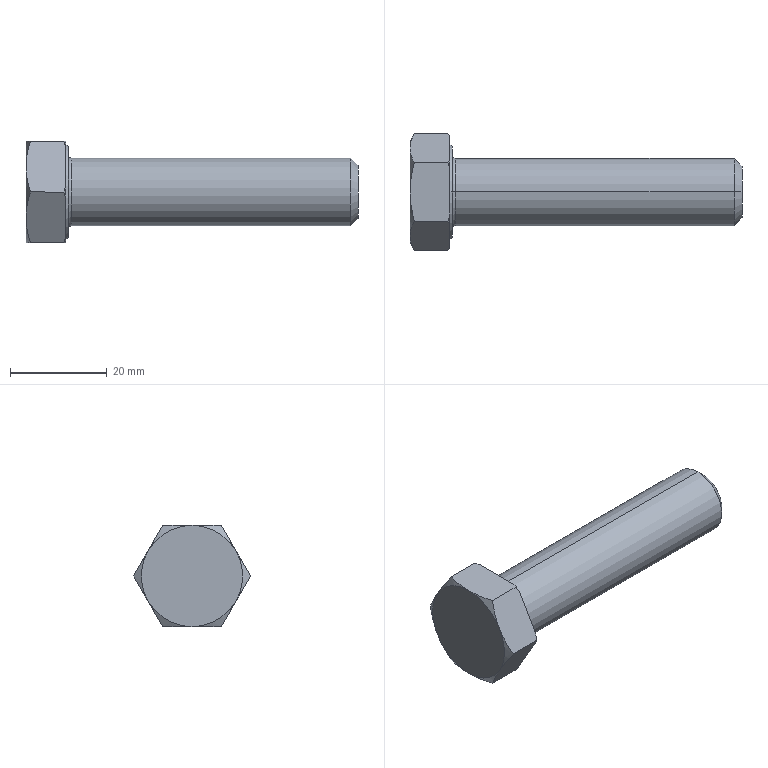Part | SolidWorks | features RevCut 4, Revolution 2, Chamfer 1, Extrusion 1, LPattern 1 | 1 solid | 30 faces | box 68.8 x 24.249 x 21 mm | volume 12486 mm3 | cone 16 | plane 10 | cylinder 2 | torus 2 | commonest cylinder face diameters 14 x2
STEP:
#1=CARTESIAN_POINT('',(9.4,0.,7.));
#2=VERTEX_POINT('',#1);
#3=CARTESIAN_POINT('',(9.4,0.,-7.));
#4=VERTEX_POINT('',#3);
#5=CARTESIAN_POINT('',(9.4,0.,0.));
#6=DIRECTION('',(-1.,0.,0.));
#7=DIRECTION('',(0.,0.,1.));
#8=AXIS2_PLACEMENT_3D('',#5,#6,#7);
#9=CIRCLE('',#8,7.);
#10=EDGE_CURVE('',#2,#4,#9,.T.);
#11=ORIENTED_EDGE('',*,*,#10,.F.);
#12=CARTESIAN_POINT('',(67.2,0.,7.));
#13=VERTEX_POINT('',#12);
#14=CARTESIAN_POINT('',(0.,0.,7.));
#15=DIRECTION('',(1.,0.,0.));
#16=VECTOR('',#15,1000.);
#17=LINE('',#14,#16);
#18=EDGE_CURVE('',#2,#13,#17,.T.);
#19=ORIENTED_EDGE('',*,*,#18,.T.);
#20=CARTESIAN_POINT('',(67.2,0.,-7.));
#21=VERTEX_POINT('',#20);
#22=CARTESIAN_POINT('',(67.2,0.,0.));
#23=DIRECTION('',(-1.,0.,0.));
#24=DIRECTION('',(0.,0.,-1.));
#25=AXIS2_PLACEMENT_3D('',#22,#23,#24);
#26=CIRCLE('',#25,7.);
#27=EDGE_CURVE('',#13,#21,#26,.T.);
#28=ORIENTED_EDGE('',*,*,#27,.T.);
#29=CARTESIAN_POINT('',(0.,0.,-7.));
#30=DIRECTION('',(1.,0.,0.));
#31=VECTOR('',#30,1000.);
#32=LINE('',#29,#31);
#33=EDGE_CURVE('',#4,#21,#32,.T.);
#34=ORIENTED_EDGE('',*,*,#33,.F.);
#35=EDGE_LOOP('',(#11,#19,#28,#34));
#36=FACE_OUTER_BOUND('',#35,.T.);
#37=CARTESIAN_POINT('',(0.,0.,0.));
#38=DIRECTION('',(1.,0.,0.));
#39=DIRECTION('',(0.,0.,-1.));
#40=AXIS2_PLACEMENT_3D('',#37,#38,#39);
#41=CYLINDRICAL_SURFACE('',#40,7.);
#42=ADVANCED_FACE('',(#36),#41,.T.);
#43=CARTESIAN_POINT('',(68.8,0.,-5.4));
#44=VERTEX_POINT('',#43);
#45=CARTESIAN_POINT('',(68.8,0.,5.4));
#46=VERTEX_POINT('',#45);
#47=CARTESIAN_POINT('',(68.8,0.,0.));
#48=DIRECTION('',(1.,0.,0.));
#49=DIRECTION('',(0.,0.,-1.));
#50=AXIS2_PLACEMENT_3D('',#47,#48,#49);
#51=CIRCLE('',#50,5.4);
#52=EDGE_CURVE('',#44,#46,#51,.T.);
#53=ORIENTED_EDGE('',*,*,#52,.F.);
#54=CARTESIAN_POINT('',(68.8,0.,-5.4));
#55=DIRECTION('',(-0.7071,0.,-0.7071));
#56=VECTOR('',#55,1000.);
#57=LINE('',#54,#56);
#58=EDGE_CURVE('',#44,#21,#57,.T.);
#59=ORIENTED_EDGE('',*,*,#58,.T.);
#60=ORIENTED_EDGE('',*,*,#27,.F.);
#61=CARTESIAN_POINT('',(68.8,0.,5.4));
#62=DIRECTION('',(-0.7071,0.,0.7071));
#63=VECTOR('',#62,1000.);
#64=LINE('',#61,#63);
#65=EDGE_CURVE('',#46,#13,#64,.T.);
#66=ORIENTED_EDGE('',*,*,#65,.F.);
#67=EDGE_LOOP('',(#53,#59,#60,#66));
#68=FACE_OUTER_BOUND('',#67,.T.);
#69=CARTESIAN_POINT('',(68.8,0.,0.));
#70=DIRECTION('',(-1.,0.,0.));
#71=DIRECTION('',(0.,0.,1.));
#72=AXIS2_PLACEMENT_3D('',#69,#70,#71);
#73=CONICAL_SURFACE('',#72,5.4,0.7854);
#74=ADVANCED_FACE('',(#68),#73,.T.);
#75=CARTESIAN_POINT('',(8.8,0.,-7.6));
#76=VERTEX_POINT('',#75);
#77=CARTESIAN_POINT('',(8.8,0.,7.6));
#78=VERTEX_POINT('',#77);
#79=CARTESIAN_POINT('',(8.8,0.,0.));
#80=DIRECTION('',(-1.,0.,0.));
#81=DIRECTION('',(0.,0.,1.));
#82=AXIS2_PLACEMENT_3D('',#79,#80,#81);
#83=CIRCLE('',#82,7.6);
#84=EDGE_CURVE('',#76,#78,#83,.T.);
#85=ORIENTED_EDGE('',*,*,#84,.F.);
#86=CARTESIAN_POINT('',(9.4,0.,-7.6));
#87=DIRECTION('',(0.,1.,0.));
#88=DIRECTION('',(0.,0.,1.));
#89=AXIS2_PLACEMENT_3D('',#86,#87,#88);
#90=CIRCLE('',#89,0.6);
#91=EDGE_CURVE('',#76,#4,#90,.T.);
#92=ORIENTED_EDGE('',*,*,#91,.T.);
#93=CARTESIAN_POINT('',(9.4,0.,0.));
#94=DIRECTION('',(-1.,0.,0.));
#95=DIRECTION('',(0.,0.,1.));
#96=AXIS2_PLACEMENT_3D('',#93,#94,#95);
#97=CIRCLE('',#96,7.);
#98=EDGE_CURVE('',#4,#2,#97,.T.);
#99=ORIENTED_EDGE('',*,*,#98,.T.);
#100=CARTESIAN_POINT('',(9.4,0.,7.6));
#101=DIRECTION('',(0.,-1.,0.));
#102=DIRECTION('',(1.,0.,0.));
#103=AXIS2_PLACEMENT_3D('',#100,#101,#102);
#104=CIRCLE('',#103,0.6);
#105=EDGE_CURVE('',#78,#2,#104,.T.);
#106=ORIENTED_EDGE('',*,*,#105,.F.);
#107=EDGE_LOOP('',(#85,#92,#99,#106));
#108=FACE_OUTER_BOUND('',#107,.T.);
#109=CARTESIAN_POINT('',(9.4,0.,0.));
#110=DIRECTION('',(-1.,0.,0.));
#111=DIRECTION('',(0.,0.,1.));
#112=AXIS2_PLACEMENT_3D('',#109,#110,#111);
#113=TOROIDAL_SURFACE('',#112,7.6,0.6);
#114=ADVANCED_FACE('',(#108),#113,.F.);
#115=CARTESIAN_POINT('',(8.8,0.,9.517));
#116=VERTEX_POINT('',#115);
#117=CARTESIAN_POINT('',(8.8,0.,-9.517));
#118=VERTEX_POINT('',#117);
#119=CARTESIAN_POINT('',(8.8,0.,0.));
#120=DIRECTION('',(-1.,0.,0.));
#121=DIRECTION('',(0.,0.,1.));
#122=AXIS2_PLACEMENT_3D('',#119,#120,#121);
#123=CIRCLE('',#122,9.517);
#124=EDGE_CURVE('',#116,#118,#123,.T.);
#125=ORIENTED_EDGE('',*,*,#124,.T.);
#126=CARTESIAN_POINT('',(8.2,0.,-9.864));
#127=VERTEX_POINT('',#126);
#128=CARTESIAN_POINT('',(8.2,0.,-9.864));
#129=DIRECTION('',(-0.866,0.,-0.5));
#130=VECTOR('',#129,1000.);
#131=LINE('',#128,#130);
#132=EDGE_CURVE('',#118,#127,#131,.T.);
#133=ORIENTED_EDGE('',*,*,#132,.T.);
#134=CARTESIAN_POINT('',(8.2,0.,9.864));
#135=VERTEX_POINT('',#134);
#136=CARTESIAN_POINT('',(8.2,0.,0.));
#137=DIRECTION('',(-1.,0.,0.));
#138=DIRECTION('',(0.,0.,1.));
#139=AXIS2_PLACEMENT_3D('',#136,#137,#138);
#140=CIRCLE('',#139,9.864);
#141=EDGE_CURVE('',#135,#127,#140,.T.);
#142=ORIENTED_EDGE('',*,*,#141,.F.);
#143=CARTESIAN_POINT('',(8.2,0.,9.864));
#144=DIRECTION('',(-0.866,0.,0.5));
#145=VECTOR('',#144,1000.);
#146=LINE('',#143,#145);
#147=EDGE_CURVE('',#116,#135,#146,.T.);
#148=ORIENTED_EDGE('',*,*,#147,.F.);
#149=EDGE_LOOP('',(#125,#133,#142,#148));
#150=FACE_OUTER_BOUND('',#149,.T.);
#151=CARTESIAN_POINT('',(8.2,0.,0.));
#152=DIRECTION('',(-1.,0.,0.));
#153=DIRECTION('',(0.,0.,1.));
#154=AXIS2_PLACEMENT_3D('',#151,#152,#153);
#155=CONICAL_SURFACE('',#154,9.864,0.5236);
#156=ADVANCED_FACE('',(#150),#155,.T.);
#157=ORIENTED_EDGE('',*,*,#124,.F.);
#158=CARTESIAN_POINT('',(8.8,0.,0.));
#159=DIRECTION('',(-1.,0.,0.));
#160=DIRECTION('',(0.,0.,1.));
#161=AXIS2_PLACEMENT_3D('',#158,#159,#160);
#162=CIRCLE('',#161,9.517);
#163=EDGE_CURVE('',#118,#116,#162,.T.);
#164=ORIENTED_EDGE('',*,*,#163,.F.);
#165=EDGE_LOOP('',(#157,#164));
#166=FACE_OUTER_BOUND('',#165,.T.);
#167=CARTESIAN_POINT('',(8.8,0.,0.));
#168=DIRECTION('',(-1.,0.,0.));
#169=DIRECTION('',(0.,0.,1.));
#170=AXIS2_PLACEMENT_3D('',#167,#168,#169);
#171=CIRCLE('',#170,7.6);
#172=EDGE_CURVE('',#78,#76,#171,.T.);
#173=ORIENTED_EDGE('',*,*,#172,.T.);
#174=ORIENTED_EDGE('',*,*,#84,.T.);
#175=EDGE_LOOP('',(#173,#174));
#176=FACE_BOUND('',#175,.T.);
#177=CARTESIAN_POINT('',(8.8,12.124,0.));
#178=DIRECTION('',(1.,0.,0.));
#179=DIRECTION('',(0.,0.,-1.));
#180=AXIS2_PLACEMENT_3D('',#177,#178,#179);
#181=PLANE('',#180);
#182=ADVANCED_FACE('',(#166,#176),#181,.T.);
#183=CARTESIAN_POINT('',(8.2,6.7,-9.395));
#184=VERTEX_POINT('',#183);
#185=CARTESIAN_POINT('',(8.2,11.486,-1.105));
#186=VERTEX_POINT('',#185);
#187=CARTESIAN_POINT('',(8.2,6.062,-10.5));
#188=DIRECTION('',(0.,0.5,0.866));
#189=VECTOR('',#188,1000.);
#190=LINE('',#187,#189);
#191=EDGE_CURVE('',#184,#186,#190,.T.);
#192=ORIENTED_EDGE('',*,*,#191,.F.);
#193=CARTESIAN_POINT('',(7.862,6.062,-10.5));
#194=VERTEX_POINT('',#193);
#195=CARTESIAN_POINT('',(7.862,6.062,-10.5));
#196=CARTESIAN_POINT('',(7.985,6.274,-10.133));
#197=CARTESIAN_POINT('',(8.098,6.487,-9.764));
#198=CARTESIAN_POINT('',(8.2,6.7,-9.395));
#199=B_SPLINE_CURVE_WITH_KNOTS('',3,(#195,#196,#197,#198),.UNSPECIFIED.,.F.,.F.,(4,4),(0.000000238,0.001312),.UNSPECIFIED.);
#200=EDGE_CURVE('',#194,#184,#199,.T.);
#201=ORIENTED_EDGE('',*,*,#200,.F.);
#202=CARTESIAN_POINT('',(0.9378,6.062,-10.5));
#203=VERTEX_POINT('',#202);
#204=CARTESIAN_POINT('',(8.8,6.062,-10.5));
#205=DIRECTION('',(-1.,0.,0.));
#206=VECTOR('',#205,1000.);
#207=LINE('',#204,#206);
#208=EDGE_CURVE('',#194,#203,#207,.T.);
#209=ORIENTED_EDGE('',*,*,#208,.T.);
#210=CARTESIAN_POINT('',(0.,9.093,-5.25));
#211=VERTEX_POINT('',#210);
#212=CARTESIAN_POINT('',(0.,9.093,-5.25));
#213=CARTESIAN_POINT('',(0.,8.836,-5.696));
#214=CARTESIAN_POINT('',(0.02217,8.578,-6.143));
#215=CARTESIAN_POINT('',(0.1079,8.066,-7.028));
#216=CARTESIAN_POINT('',(0.1715,7.813,-7.468));
#217=CARTESIAN_POINT('',(0.4165,7.056,-8.779));
#218=CARTESIAN_POINT('',(0.6523,6.557,-9.643));
#219=CARTESIAN_POINT('',(0.9378,6.062,-10.5));
#220=B_SPLINE_CURVE_WITH_KNOTS('',3,(#212,#213,#214,#215,#216,#217,#218,#219),.UNSPECIFIED.,.F.,.F.,(4,2,2,4),(0.006134,0.007662,0.00919,0.01225),.UNSPECIFIED.);
#221=EDGE_CURVE('',#211,#203,#220,.T.);
#222=ORIENTED_EDGE('',*,*,#221,.F.);
#223=CARTESIAN_POINT('',(0.9378,12.124,0.));
#224=VERTEX_POINT('',#223);
#225=CARTESIAN_POINT('',(0.9378,12.124,0.));
#226=CARTESIAN_POINT('',(0.6515,11.629,-0.8588));
#227=CARTESIAN_POINT('',(0.4157,11.129,-1.724));
#228=CARTESIAN_POINT('',(0.08938,10.12,-3.472));
#229=CARTESIAN_POINT('',(0.,9.61,-4.356));
#230=CARTESIAN_POINT('',(0.,9.093,-5.25));
#231=B_SPLINE_CURVE_WITH_KNOTS('',3,(#225,#226,#227,#228,#229,#230),.UNSPECIFIED.,.F.,.F.,(4,2,4),(0.000000238,0.003067,0.006134),.UNSPECIFIED.);
#232=EDGE_CURVE('',#224,#211,#231,.T.);
#233=ORIENTED_EDGE('',*,*,#232,.F.);
#234=CARTESIAN_POINT('',(7.862,12.124,0.));
#235=VERTEX_POINT('',#234);
#236=CARTESIAN_POINT('',(8.8,12.124,0.));
#237=DIRECTION('',(-1.,0.,0.));
#238=VECTOR('',#237,1000.);
#239=LINE('',#236,#238);
#240=EDGE_CURVE('',#235,#224,#239,.T.);
#241=ORIENTED_EDGE('',*,*,#240,.F.);
#242=CARTESIAN_POINT('',(8.2,11.486,-1.105));
#243=CARTESIAN_POINT('',(8.098,11.7,-0.7354));
#244=CARTESIAN_POINT('',(7.985,11.912,-0.3671));
#245=CARTESIAN_POINT('',(7.862,12.124,0.));
#246=B_SPLINE_CURVE_WITH_KNOTS('',3,(#242,#243,#244,#245),.UNSPECIFIED.,.F.,.F.,(4,4),(0.01094,0.01225),.UNSPECIFIED.);
#247=EDGE_CURVE('',#186,#235,#246,.T.);
#248=ORIENTED_EDGE('',*,*,#247,.F.);
#249=EDGE_LOOP('',(#192,#201,#209,#222,#233,#241,#248));
#250=FACE_OUTER_BOUND('',#249,.T.);
#251=CARTESIAN_POINT('',(8.8,6.062,-10.5));
#252=DIRECTION('',(0.,-0.866,0.5));
#253=DIRECTION('',(0.,-0.5,-0.866));
#254=AXIS2_PLACEMENT_3D('',#251,#252,#253);
#255=PLANE('',#254);
#256=ADVANCED_FACE('',(#250),#255,.F.);
#257=CARTESIAN_POINT('',(8.2,11.486,1.105));
#258=VERTEX_POINT('',#257);
#259=CARTESIAN_POINT('',(8.2,6.7,9.395));
#260=VERTEX_POINT('',#259);
#261=CARTESIAN_POINT('',(8.2,12.124,0.));
#262=DIRECTION('',(0.,-0.5,0.866));
#263=VECTOR('',#262,1000.);
#264=LINE('',#261,#263);
#265=EDGE_CURVE('',#258,#260,#264,.T.);
#266=ORIENTED_EDGE('',*,*,#265,.F.);
#267=CARTESIAN_POINT('',(7.862,12.124,0.));
#268=CARTESIAN_POINT('',(7.985,11.912,0.3672));
#269=CARTESIAN_POINT('',(8.098,11.7,0.7356));
#270=CARTESIAN_POINT('',(8.2,11.486,1.105));
#271=B_SPLINE_CURVE_WITH_KNOTS('',3,(#267,#268,#269,#270),.UNSPECIFIED.,.F.,.F.,(4,4),(0.000000238,0.001312),.UNSPECIFIED.);
#272=EDGE_CURVE('',#235,#258,#271,.T.);
#273=ORIENTED_EDGE('',*,*,#272,.F.);
#274=ORIENTED_EDGE('',*,*,#240,.T.);
#275=CARTESIAN_POINT('',(0.,9.093,5.25));
#276=VERTEX_POINT('',#275);
#277=CARTESIAN_POINT('',(0.,9.093,5.25));
#278=CARTESIAN_POINT('',(0.,9.351,4.804));
#279=CARTESIAN_POINT('',(0.02217,9.609,4.357));
#280=CARTESIAN_POINT('',(0.1079,10.12,3.472));
#281=CARTESIAN_POINT('',(0.1715,10.374,3.032));
#282=CARTESIAN_POINT('',(0.4165,11.131,1.721));
#283=CARTESIAN_POINT('',(0.6523,11.63,0.8567));
#284=CARTESIAN_POINT('',(0.9378,12.124,0.));
#285=B_SPLINE_CURVE_WITH_KNOTS('',3,(#277,#278,#279,#280,#281,#282,#283,#284),.UNSPECIFIED.,.F.,.F.,(4,2,2,4),(0.006134,0.007662,0.00919,0.01225),.UNSPECIFIED.);
#286=EDGE_CURVE('',#276,#224,#285,.T.);
#287=ORIENTED_EDGE('',*,*,#286,.F.);
#288=CARTESIAN_POINT('',(0.9378,6.062,10.5));
#289=VERTEX_POINT('',#288);
#290=CARTESIAN_POINT('',(0.9378,6.062,10.5));
#291=CARTESIAN_POINT('',(0.6515,6.558,9.641));
#292=CARTESIAN_POINT('',(0.4157,7.057,8.776));
#293=CARTESIAN_POINT('',(0.08938,8.067,7.028));
#294=CARTESIAN_POINT('',(0.,8.577,6.144));
#295=CARTESIAN_POINT('',(0.,9.093,5.25));
#296=B_SPLINE_CURVE_WITH_KNOTS('',3,(#290,#291,#292,#293,#294,#295),.UNSPECIFIED.,.F.,.F.,(4,2,4),(0.000000238,0.003067,0.006134),.UNSPECIFIED.);
#297=EDGE_CURVE('',#289,#276,#296,.T.);
#298=ORIENTED_EDGE('',*,*,#297,.F.);
#299=CARTESIAN_POINT('',(7.862,6.062,10.5));
#300=VERTEX_POINT('',#299);
#301=CARTESIAN_POINT('',(8.8,6.062,10.5));
#302=DIRECTION('',(-1.,0.,0.));
#303=VECTOR('',#302,1000.);
#304=LINE('',#301,#303);
#305=EDGE_CURVE('',#300,#289,#304,.T.);
#306=ORIENTED_EDGE('',*,*,#305,.F.);
#307=CARTESIAN_POINT('',(8.2,6.7,9.395));
#308=CARTESIAN_POINT('',(8.098,6.487,9.765));
#309=CARTESIAN_POINT('',(7.985,6.274,10.133));
#310=CARTESIAN_POINT('',(7.862,6.062,10.5));
#311=B_SPLINE_CURVE_WITH_KNOTS('',3,(#307,#308,#309,#310),.UNSPECIFIED.,.F.,.F.,(4,4),(0.01094,0.01225),.UNSPECIFIED.);
#312=EDGE_CURVE('',#260,#300,#311,.T.);
#313=ORIENTED_EDGE('',*,*,#312,.F.);
#314=EDGE_LOOP('',(#266,#273,#274,#287,#298,#306,#313));
#315=FACE_OUTER_BOUND('',#314,.T.);
#316=CARTESIAN_POINT('',(8.8,12.124,0.));
#317=DIRECTION('',(0.,-0.866,-0.5));
#318=DIRECTION('',(0.,0.5,-0.866));
#319=AXIS2_PLACEMENT_3D('',#316,#317,#318);
#320=PLANE('',#319);
#321=ADVANCED_FACE('',(#315),#320,.F.);
#322=CARTESIAN_POINT('',(8.2,4.786,10.5));
#323=VERTEX_POINT('',#322);
#324=CARTESIAN_POINT('',(8.2,-4.786,10.5));
#325=VERTEX_POINT('',#324);
#326=CARTESIAN_POINT('',(8.2,6.062,10.5));
#327=DIRECTION('',(0.,-1.,0.));
#328=VECTOR('',#327,1000.);
#329=LINE('',#326,#328);
#330=EDGE_CURVE('',#323,#325,#329,.T.);
#331=ORIENTED_EDGE('',*,*,#330,.F.);
#332=CARTESIAN_POINT('',(7.862,6.062,10.5));
#333=CARTESIAN_POINT('',(7.984,5.639,10.5));
#334=CARTESIAN_POINT('',(8.097,5.214,10.5));
#335=CARTESIAN_POINT('',(8.2,4.786,10.5));
#336=B_SPLINE_CURVE_WITH_KNOTS('',3,(#332,#333,#334,#335),.UNSPECIFIED.,.F.,.F.,(4,4),(0.02875,0.03008),.UNSPECIFIED.);
#337=EDGE_CURVE('',#300,#323,#336,.T.);
#338=ORIENTED_EDGE('',*,*,#337,.F.);
#339=ORIENTED_EDGE('',*,*,#305,.T.);
#340=CARTESIAN_POINT('',(0.,0.,10.5));
#341=VERTEX_POINT('',#340);
#342=CARTESIAN_POINT('',(0.,0.,10.5));
#343=CARTESIAN_POINT('',(0.,0.5133,10.5));
#344=CARTESIAN_POINT('',(0.02195,1.03,10.5));
#345=CARTESIAN_POINT('',(0.1087,2.061,10.5));
#346=CARTESIAN_POINT('',(0.1729,2.572,10.5));
#347=CARTESIAN_POINT('',(0.4192,4.089,10.5));
#348=CARTESIAN_POINT('',(0.6548,5.082,10.5));
#349=CARTESIAN_POINT('',(0.9378,6.062,10.5));
#350=B_SPLINE_CURVE_WITH_KNOTS('',3,(#342,#343,#344,#345,#346,#347,#348,#349),.UNSPECIFIED.,.F.,.F.,(4,2,2,4),(0.0174,0.01894,0.02047,0.02354),.UNSPECIFIED.);
#351=EDGE_CURVE('',#341,#289,#350,.T.);
#352=ORIENTED_EDGE('',*,*,#351,.F.);
#353=CARTESIAN_POINT('',(0.9378,-6.062,10.5));
#354=VERTEX_POINT('',#353);
#355=CARTESIAN_POINT('',(0.9378,-6.062,10.5));
#356=CARTESIAN_POINT('',(0.6528,-5.075,10.5));
#357=CARTESIAN_POINT('',(0.4144,-4.066,10.5));
#358=CARTESIAN_POINT('',(0.08826,-2.044,10.5));
#359=CARTESIAN_POINT('',(0.,-1.026,10.5));
#360=CARTESIAN_POINT('',(0.,0.,10.5));
#361=B_SPLINE_CURVE_WITH_KNOTS('',3,(#355,#356,#357,#358,#359,#360),.UNSPECIFIED.,.F.,.F.,(4,2,4),(0.01126,0.01433,0.0174),.UNSPECIFIED.);
#362=EDGE_CURVE('',#354,#341,#361,.T.);
#363=ORIENTED_EDGE('',*,*,#362,.F.);
#364=CARTESIAN_POINT('',(7.862,-6.062,10.5));
#365=VERTEX_POINT('',#364);
#366=CARTESIAN_POINT('',(8.8,-6.062,10.5));
#367=DIRECTION('',(-1.,0.,0.));
#368=VECTOR('',#367,1000.);
#369=LINE('',#366,#368);
#370=EDGE_CURVE('',#365,#354,#369,.T.);
#371=ORIENTED_EDGE('',*,*,#370,.F.);
#372=CARTESIAN_POINT('',(8.2,-4.786,10.5));
#373=CARTESIAN_POINT('',(8.097,-5.215,10.5));
#374=CARTESIAN_POINT('',(7.984,-5.64,10.5));
#375=CARTESIAN_POINT('',(7.862,-6.062,10.5));
#376=B_SPLINE_CURVE_WITH_KNOTS('',3,(#372,#373,#374,#375),.UNSPECIFIED.,.F.,.F.,(4,4),(0.03972,0.04103),.UNSPECIFIED.);
#377=EDGE_CURVE('',#325,#365,#376,.T.);
#378=ORIENTED_EDGE('',*,*,#377,.F.);
#379=EDGE_LOOP('',(#331,#338,#339,#352,#363,#371,#378));
#380=FACE_OUTER_BOUND('',#379,.T.);
#381=CARTESIAN_POINT('',(8.8,6.062,10.5));
#382=DIRECTION('',(0.,0.,-1.));
#383=DIRECTION('',(0.,1.,0.));
#384=AXIS2_PLACEMENT_3D('',#381,#382,#383);
#385=PLANE('',#384);
#386=ADVANCED_FACE('',(#380),#385,.F.);
#387=CARTESIAN_POINT('',(8.2,-6.7,9.395));
#388=VERTEX_POINT('',#387);
#389=CARTESIAN_POINT('',(8.2,-11.486,1.105));
#390=VERTEX_POINT('',#389);
#391=CARTESIAN_POINT('',(8.2,-12.124,0.));
#392=DIRECTION('',(0.,-0.5,-0.866));
#393=VECTOR('',#392,1000.);
#394=LINE('',#391,#393);
#395=EDGE_CURVE('',#388,#390,#394,.T.);
#396=ORIENTED_EDGE('',*,*,#395,.F.);
#397=CARTESIAN_POINT('',(7.862,-6.062,10.5));
#398=CARTESIAN_POINT('',(7.985,-6.274,10.133));
#399=CARTESIAN_POINT('',(8.098,-6.487,9.764));
#400=CARTESIAN_POINT('',(8.2,-6.7,9.395));
#401=B_SPLINE_CURVE_WITH_KNOTS('',3,(#397,#398,#399,#400),.UNSPECIFIED.,.F.,.F.,(4,4),(0.000000238,0.001312),.UNSPECIFIED.);
#402=EDGE_CURVE('',#365,#388,#401,.T.);
#403=ORIENTED_EDGE('',*,*,#402,.F.);
#404=ORIENTED_EDGE('',*,*,#370,.T.);
#405=CARTESIAN_POINT('',(0.,-9.093,5.25));
#406=VERTEX_POINT('',#405);
#407=CARTESIAN_POINT('',(0.,-9.093,5.25));
#408=CARTESIAN_POINT('',(0.,-8.836,5.696));
#409=CARTESIAN_POINT('',(0.02217,-8.578,6.143));
#410=CARTESIAN_POINT('',(0.1079,-8.066,7.028));
#411=CARTESIAN_POINT('',(0.1715,-7.813,7.468));
#412=CARTESIAN_POINT('',(0.4165,-7.056,8.779));
#413=CARTESIAN_POINT('',(0.6523,-6.557,9.643));
#414=CARTESIAN_POINT('',(0.9378,-6.062,10.5));
#415=B_SPLINE_CURVE_WITH_KNOTS('',3,(#407,#408,#409,#410,#411,#412,#413,#414),.UNSPECIFIED.,.F.,.F.,(4,2,2,4),(0.006134,0.007662,0.00919,0.01225),.UNSPECIFIED.);
#416=EDGE_CURVE('',#406,#354,#415,.T.);
#417=ORIENTED_EDGE('',*,*,#416,.F.);
#418=CARTESIAN_POINT('',(0.9378,-12.124,0.));
#419=VERTEX_POINT('',#418);
#420=CARTESIAN_POINT('',(0.9378,-12.124,0.));
#421=CARTESIAN_POINT('',(0.6515,-11.629,0.8588));
#422=CARTESIAN_POINT('',(0.4157,-11.129,1.724));
#423=CARTESIAN_POINT('',(0.08938,-10.12,3.472));
#424=CARTESIAN_POINT('',(0.,-9.61,4.356));
#425=CARTESIAN_POINT('',(0.,-9.093,5.25));
#426=B_SPLINE_CURVE_WITH_KNOTS('',3,(#420,#421,#422,#423,#424,#425),.UNSPECIFIED.,.F.,.F.,(4,2,4),(0.000000238,0.003067,0.006134),.UNSPECIFIED.);
#427=EDGE_CURVE('',#419,#406,#426,.T.);
#428=ORIENTED_EDGE('',*,*,#427,.F.);
#429=CARTESIAN_POINT('',(7.862,-12.124,0.));
#430=VERTEX_POINT('',#429);
#431=CARTESIAN_POINT('',(8.8,-12.124,0.));
#432=DIRECTION('',(-1.,0.,0.));
#433=VECTOR('',#432,1000.);
#434=LINE('',#431,#433);
#435=EDGE_CURVE('',#430,#419,#434,.T.);
#436=ORIENTED_EDGE('',*,*,#435,.F.);
#437=CARTESIAN_POINT('',(8.2,-11.486,1.105));
#438=CARTESIAN_POINT('',(8.098,-11.7,0.7354));
#439=CARTESIAN_POINT('',(7.985,-11.912,0.3671));
#440=CARTESIAN_POINT('',(7.862,-12.124,0.));
#441=B_SPLINE_CURVE_WITH_KNOTS('',3,(#437,#438,#439,#440),.UNSPECIFIED.,.F.,.F.,(4,4),(0.01094,0.01225),.UNSPECIFIED.);
#442=EDGE_CURVE('',#390,#430,#441,.T.);
#443=ORIENTED_EDGE('',*,*,#442,.F.);
#444=EDGE_LOOP('',(#396,#403,#404,#417,#428,#436,#443));
#445=FACE_OUTER_BOUND('',#444,.T.);
#446=CARTESIAN_POINT('',(8.8,-12.124,0.));
#447=DIRECTION('',(0.,0.866,-0.5));
#448=DIRECTION('',(0.,0.5,0.866));
#449=AXIS2_PLACEMENT_3D('',#446,#447,#448);
#450=PLANE('',#449);
#451=ADVANCED_FACE('',(#445),#450,.F.);
#452=CARTESIAN_POINT('',(8.2,-11.486,-1.105));
#453=VERTEX_POINT('',#452);
#454=CARTESIAN_POINT('',(8.2,-6.7,-9.395));
#455=VERTEX_POINT('',#454);
#456=CARTESIAN_POINT('',(8.2,-6.062,-10.5));
#457=DIRECTION('',(0.,0.5,-0.866));
#458=VECTOR('',#457,1000.);
#459=LINE('',#456,#458);
#460=EDGE_CURVE('',#453,#455,#459,.T.);
#461=ORIENTED_EDGE('',*,*,#460,.F.);
#462=CARTESIAN_POINT('',(7.862,-12.124,0.));
#463=CARTESIAN_POINT('',(7.985,-11.912,-0.3672));
#464=CARTESIAN_POINT('',(8.098,-11.7,-0.7356));
#465=CARTESIAN_POINT('',(8.2,-11.486,-1.105));
#466=B_SPLINE_CURVE_WITH_KNOTS('',3,(#462,#463,#464,#465),.UNSPECIFIED.,.F.,.F.,(4,4),(0.000000238,0.001312),.UNSPECIFIED.);
#467=EDGE_CURVE('',#430,#453,#466,.T.);
#468=ORIENTED_EDGE('',*,*,#467,.F.);
#469=ORIENTED_EDGE('',*,*,#435,.T.);
#470=CARTESIAN_POINT('',(0.,-9.093,-5.25));
#471=VERTEX_POINT('',#470);
#472=CARTESIAN_POINT('',(0.,-9.093,-5.25));
#473=CARTESIAN_POINT('',(0.,-9.351,-4.804));
#474=CARTESIAN_POINT('',(0.02217,-9.609,-4.357));
#475=CARTESIAN_POINT('',(0.1079,-10.12,-3.472));
#476=CARTESIAN_POINT('',(0.1715,-10.374,-3.032));
#477=CARTESIAN_POINT('',(0.4165,-11.131,-1.721));
#478=CARTESIAN_POINT('',(0.6523,-11.63,-0.8567));
#479=CARTESIAN_POINT('',(0.9378,-12.124,0.));
#480=B_SPLINE_CURVE_WITH_KNOTS('',3,(#472,#473,#474,#475,#476,#477,#478,#479),.UNSPECIFIED.,.F.,.F.,(4,2,2,4),(0.006134,0.007662,0.00919,0.01225),.UNSPECIFIED.);
#481=EDGE_CURVE('',#471,#419,#480,.T.);
#482=ORIENTED_EDGE('',*,*,#481,.F.);
#483=CARTESIAN_POINT('',(0.9378,-6.062,-10.5));
#484=VERTEX_POINT('',#483);
#485=CARTESIAN_POINT('',(0.9378,-6.062,-10.5));
#486=CARTESIAN_POINT('',(0.6515,-6.558,-9.641));
#487=CARTESIAN_POINT('',(0.4157,-7.057,-8.776));
#488=CARTESIAN_POINT('',(0.08938,-8.067,-7.028));
#489=CARTESIAN_POINT('',(0.,-8.577,-6.144));
#490=CARTESIAN_POINT('',(0.,-9.093,-5.25));
#491=B_SPLINE_CURVE_WITH_KNOTS('',3,(#485,#486,#487,#488,#489,#490),.UNSPECIFIED.,.F.,.F.,(4,2,4),(0.000000238,0.003067,0.006134),.UNSPECIFIED.);
#492=EDGE_CURVE('',#484,#471,#491,.T.);
#493=ORIENTED_EDGE('',*,*,#492,.F.);
#494=CARTESIAN_POINT('',(7.862,-6.062,-10.5));
#495=VERTEX_POINT('',#494);
#496=CARTESIAN_POINT('',(8.8,-6.062,-10.5));
#497=DIRECTION('',(-1.,0.,0.));
#498=VECTOR('',#497,1000.);
#499=LINE('',#496,#498);
#500=EDGE_CURVE('',#495,#484,#499,.T.);
#501=ORIENTED_EDGE('',*,*,#500,.F.);
#502=CARTESIAN_POINT('',(8.2,-6.7,-9.395));
#503=CARTESIAN_POINT('',(8.098,-6.487,-9.765));
#504=CARTESIAN_POINT('',(7.985,-6.274,-10.133));
#505=CARTESIAN_POINT('',(7.862,-6.062,-10.5));
#506=B_SPLINE_CURVE_WITH_KNOTS('',3,(#502,#503,#504,#505),.UNSPECIFIED.,.F.,.F.,(4,4),(0.01094,0.01225),.UNSPECIFIED.);
#507=EDGE_CURVE('',#455,#495,#506,.T.);
#508=ORIENTED_EDGE('',*,*,#507,.F.);
#509=EDGE_LOOP('',(#461,#468,#469,#482,#493,#501,#508));
#510=FACE_OUTER_BOUND('',#509,.T.);
#511=CARTESIAN_POINT('',(8.8,-6.062,-10.5));
#512=DIRECTION('',(0.,0.866,0.5));
#513=DIRECTION('',(0.,-0.5,0.866));
#514=AXIS2_PLACEMENT_3D('',#511,#512,#513);
#515=PLANE('',#514);
#516=ADVANCED_FACE('',(#510),#515,.F.);
#517=CARTESIAN_POINT('',(8.2,-4.786,-10.5));
#518=VERTEX_POINT('',#517);
#519=CARTESIAN_POINT('',(8.2,4.786,-10.5));
#520=VERTEX_POINT('',#519);
#521=CARTESIAN_POINT('',(8.2,6.062,-10.5));
#522=DIRECTION('',(0.,1.,0.));
#523=VECTOR('',#522,1000.);
#524=LINE('',#521,#523);
#525=EDGE_CURVE('',#518,#520,#524,.T.);
#526=ORIENTED_EDGE('',*,*,#525,.F.);
#527=CARTESIAN_POINT('',(7.862,-6.062,-10.5));
#528=CARTESIAN_POINT('',(7.984,-5.64,-10.5));
#529=CARTESIAN_POINT('',(8.097,-5.215,-10.5));
#530=CARTESIAN_POINT('',(8.2,-4.786,-10.5));
#531=B_SPLINE_CURVE_WITH_KNOTS('',3,(#527,#528,#529,#530),.UNSPECIFIED.,.F.,.F.,(4,4),(0.01126,0.01258),.UNSPECIFIED.);
#532=EDGE_CURVE('',#495,#518,#531,.T.);
#533=ORIENTED_EDGE('',*,*,#532,.F.);
#534=ORIENTED_EDGE('',*,*,#500,.T.);
#535=CARTESIAN_POINT('',(0.,0.,-10.5));
#536=VERTEX_POINT('',#535);
#537=CARTESIAN_POINT('',(0.,0.,-10.5));
#538=CARTESIAN_POINT('',(0.,-1.026,-10.5));
#539=CARTESIAN_POINT('',(0.08826,-2.044,-10.5));
#540=CARTESIAN_POINT('',(0.4144,-4.066,-10.5));
#541=CARTESIAN_POINT('',(0.6528,-5.075,-10.5));
#542=CARTESIAN_POINT('',(0.9378,-6.062,-10.5));
#543=B_SPLINE_CURVE_WITH_KNOTS('',3,(#537,#538,#539,#540,#541,#542),.UNSPECIFIED.,.F.,.F.,(4,2,4),(0.03489,0.03796,0.04103),.UNSPECIFIED.);
#544=EDGE_CURVE('',#536,#484,#543,.T.);
#545=ORIENTED_EDGE('',*,*,#544,.F.);
#546=CARTESIAN_POINT('',(0.9378,6.062,-10.5));
#547=CARTESIAN_POINT('',(0.6548,5.082,-10.5));
#548=CARTESIAN_POINT('',(0.4192,4.089,-10.5));
#549=CARTESIAN_POINT('',(0.1729,2.572,-10.5));
#550=CARTESIAN_POINT('',(0.1087,2.061,-10.5));
#551=CARTESIAN_POINT('',(0.02195,1.03,-10.5));
#552=CARTESIAN_POINT('',(0.,0.5133,-10.5));
#553=CARTESIAN_POINT('',(0.,0.,-10.5));
#554=B_SPLINE_CURVE_WITH_KNOTS('',3,(#546,#547,#548,#549,#550,#551,#552,#553),.UNSPECIFIED.,.F.,.F.,(4,2,2,4),(0.02875,0.03182,0.03336,0.03489),.UNSPECIFIED.);
#555=EDGE_CURVE('',#203,#536,#554,.T.);
#556=ORIENTED_EDGE('',*,*,#555,.F.);
#557=ORIENTED_EDGE('',*,*,#208,.F.);
#558=CARTESIAN_POINT('',(8.2,4.786,-10.5));
#559=CARTESIAN_POINT('',(8.097,5.214,-10.5));
#560=CARTESIAN_POINT('',(7.984,5.639,-10.5));
#561=CARTESIAN_POINT('',(7.862,6.062,-10.5));
#562=B_SPLINE_CURVE_WITH_KNOTS('',3,(#558,#559,#560,#561),.UNSPECIFIED.,.F.,.F.,(4,4),(0.02222,0.02354),.UNSPECIFIED.);
#563=EDGE_CURVE('',#520,#194,#562,.T.);
#564=ORIENTED_EDGE('',*,*,#563,.F.);
#565=EDGE_LOOP('',(#526,#533,#534,#545,#556,#557,#564));
#566=FACE_OUTER_BOUND('',#565,.T.);
#567=CARTESIAN_POINT('',(8.8,6.062,-10.5));
#568=DIRECTION('',(0.,0.,1.));
#569=DIRECTION('',(1.,0.,0.));
#570=AXIS2_PLACEMENT_3D('',#567,#568,#569);
#571=PLANE('',#570);
#572=ADVANCED_FACE('',(#566),#571,.F.);
#573=ORIENTED_EDGE('',*,*,#532,.T.);
#574=CARTESIAN_POINT('',(8.2,0.,0.));
#575=DIRECTION('',(-1.,0.,0.));
#576=DIRECTION('',(0.,0.,-1.));
#577=AXIS2_PLACEMENT_3D('',#574,#575,#576);
#578=CIRCLE('',#577,11.539);
#579=EDGE_CURVE('',#518,#455,#578,.T.);
#580=ORIENTED_EDGE('',*,*,#579,.T.);
#581=ORIENTED_EDGE('',*,*,#507,.T.);
#582=EDGE_LOOP('',(#573,#580,#581));
#583=FACE_OUTER_BOUND('',#582,.T.);
#584=CARTESIAN_POINT('',(4.975,0.,0.));
#585=DIRECTION('',(-1.,0.,0.));
#586=DIRECTION('',(0.,0.,1.));
#587=AXIS2_PLACEMENT_3D('',#584,#585,#586);
#588=CONICAL_SURFACE('',#587,17.124,1.047);
#589=ADVANCED_FACE('',(#583),#588,.T.);
#590=ORIENTED_EDGE('',*,*,#467,.T.);
#591=CARTESIAN_POINT('',(8.2,0.,0.));
#592=DIRECTION('',(-1.,0.,0.));
#593=DIRECTION('',(0.,0.,-1.));
#594=AXIS2_PLACEMENT_3D('',#591,#592,#593);
#595=CIRCLE('',#594,11.539);
#596=EDGE_CURVE('',#453,#390,#595,.T.);
#597=ORIENTED_EDGE('',*,*,#596,.T.);
#598=ORIENTED_EDGE('',*,*,#442,.T.);
#599=EDGE_LOOP('',(#590,#597,#598));
#600=FACE_OUTER_BOUND('',#599,.T.);
#601=CARTESIAN_POINT('',(4.975,0.,0.));
#602=DIRECTION('',(-1.,0.,0.));
#603=DIRECTION('',(0.,0.,1.));
#604=AXIS2_PLACEMENT_3D('',#601,#602,#603);
#605=CONICAL_SURFACE('',#604,17.124,1.047);
#606=ADVANCED_FACE('',(#600),#605,.T.);
#607=ORIENTED_EDGE('',*,*,#402,.T.);
#608=CARTESIAN_POINT('',(8.2,0.,0.));
#609=DIRECTION('',(-1.,0.,0.));
#610=DIRECTION('',(0.,0.,-1.));
#611=AXIS2_PLACEMENT_3D('',#608,#609,#610);
#612=CIRCLE('',#611,11.539);
#613=EDGE_CURVE('',#388,#325,#612,.T.);
#614=ORIENTED_EDGE('',*,*,#613,.T.);
#615=ORIENTED_EDGE('',*,*,#377,.T.);
#616=EDGE_LOOP('',(#607,#614,#615));
#617=FACE_OUTER_BOUND('',#616,.T.);
#618=CARTESIAN_POINT('',(4.975,0.,0.));
#619=DIRECTION('',(-1.,0.,0.));
#620=DIRECTION('',(0.,0.,1.));
#621=AXIS2_PLACEMENT_3D('',#618,#619,#620);
#622=CONICAL_SURFACE('',#621,17.124,1.047);
#623=ADVANCED_FACE('',(#617),#622,.T.);
#624=ORIENTED_EDGE('',*,*,#337,.T.);
#625=CARTESIAN_POINT('',(8.2,0.,0.));
#626=DIRECTION('',(-1.,0.,0.));
#627=DIRECTION('',(0.,0.,-1.));
#628=AXIS2_PLACEMENT_3D('',#625,#626,#627);
#629=CIRCLE('',#628,11.539);
#630=EDGE_CURVE('',#323,#260,#629,.T.);
#631=ORIENTED_EDGE('',*,*,#630,.T.);
#632=ORIENTED_EDGE('',*,*,#312,.T.);
#633=EDGE_LOOP('',(#624,#631,#632));
#634=FACE_OUTER_BOUND('',#633,.T.);
#635=CARTESIAN_POINT('',(4.975,0.,0.));
#636=DIRECTION('',(-1.,0.,0.));
#637=DIRECTION('',(0.,0.,1.));
#638=AXIS2_PLACEMENT_3D('',#635,#636,#637);
#639=CONICAL_SURFACE('',#638,17.124,1.047);
#640=ADVANCED_FACE('',(#634),#639,.T.);
#641=ORIENTED_EDGE('',*,*,#272,.T.);
#642=CARTESIAN_POINT('',(8.2,0.,0.));
#643=DIRECTION('',(-1.,0.,0.));
#644=DIRECTION('',(0.,0.,-1.));
#645=AXIS2_PLACEMENT_3D('',#642,#643,#644);
#646=CIRCLE('',#645,11.539);
#647=EDGE_CURVE('',#258,#186,#646,.T.);
#648=ORIENTED_EDGE('',*,*,#647,.T.);
#649=ORIENTED_EDGE('',*,*,#247,.T.);
#650=EDGE_LOOP('',(#641,#648,#649));
#651=FACE_OUTER_BOUND('',#650,.T.);
#652=CARTESIAN_POINT('',(4.975,0.,0.));
#653=DIRECTION('',(-1.,0.,0.));
#654=DIRECTION('',(0.,0.,1.));
#655=AXIS2_PLACEMENT_3D('',#652,#653,#654);
#656=CONICAL_SURFACE('',#655,17.124,1.047);
#657=ADVANCED_FACE('',(#651),#656,.T.);
#658=ORIENTED_EDGE('',*,*,#200,.T.);
#659=CARTESIAN_POINT('',(8.2,0.,0.));
#660=DIRECTION('',(-1.,0.,0.));
#661=DIRECTION('',(0.,0.,-1.));
#662=AXIS2_PLACEMENT_3D('',#659,#660,#661);
#663=CIRCLE('',#662,11.539);
#664=EDGE_CURVE('',#184,#520,#663,.T.);
#665=ORIENTED_EDGE('',*,*,#664,.T.);
#666=ORIENTED_EDGE('',*,*,#563,.T.);
#667=EDGE_LOOP('',(#658,#665,#666));
#668=FACE_OUTER_BOUND('',#667,.T.);
#669=CARTESIAN_POINT('',(4.975,0.,0.));
#670=DIRECTION('',(-1.,0.,0.));
#671=DIRECTION('',(0.,0.,1.));
#672=AXIS2_PLACEMENT_3D('',#669,#670,#671);
#673=CONICAL_SURFACE('',#672,17.124,1.047);
#674=ADVANCED_FACE('',(#668),#673,.T.);
#675=ORIENTED_EDGE('',*,*,#492,.T.);
#676=CARTESIAN_POINT('',(0.,0.,0.));
#677=DIRECTION('',(1.,0.,0.));
#678=DIRECTION('',(0.,0.,-1.));
#679=AXIS2_PLACEMENT_3D('',#676,#677,#678);
#680=CIRCLE('',#679,10.5);
#681=EDGE_CURVE('',#471,#536,#680,.T.);
#682=ORIENTED_EDGE('',*,*,#681,.T.);
#683=ORIENTED_EDGE('',*,*,#544,.T.);
#684=EDGE_LOOP('',(#675,#682,#683));
#685=FACE_OUTER_BOUND('',#684,.T.);
#686=CARTESIAN_POINT('',(0.,0.,0.));
#687=DIRECTION('',(1.,0.,0.));
#688=DIRECTION('',(0.,0.,-1.));
#689=AXIS2_PLACEMENT_3D('',#686,#687,#688);
#690=CONICAL_SURFACE('',#689,10.5,1.047);
#691=ADVANCED_FACE('',(#685),#690,.T.);
#692=ORIENTED_EDGE('',*,*,#427,.T.);
#693=CARTESIAN_POINT('',(0.,0.,0.));
#694=DIRECTION('',(1.,0.,0.));
#695=DIRECTION('',(0.,0.,-1.));
#696=AXIS2_PLACEMENT_3D('',#693,#694,#695);
#697=CIRCLE('',#696,10.5);
#698=EDGE_CURVE('',#406,#471,#697,.T.);
#699=ORIENTED_EDGE('',*,*,#698,.T.);
#700=ORIENTED_EDGE('',*,*,#481,.T.);
#701=EDGE_LOOP('',(#692,#699,#700));
#702=FACE_OUTER_BOUND('',#701,.T.);
#703=CARTESIAN_POINT('',(0.,0.,0.));
#704=DIRECTION('',(1.,0.,0.));
#705=DIRECTION('',(0.,0.,-1.));
#706=AXIS2_PLACEMENT_3D('',#703,#704,#705);
#707=CONICAL_SURFACE('',#706,10.5,1.047);
#708=ADVANCED_FACE('',(#702),#707,.T.);
#709=ORIENTED_EDGE('',*,*,#362,.T.);
#710=CARTESIAN_POINT('',(0.,0.,0.));
#711=DIRECTION('',(1.,0.,0.));
#712=DIRECTION('',(0.,0.,-1.));
#713=AXIS2_PLACEMENT_3D('',#710,#711,#712);
#714=CIRCLE('',#713,10.5);
#715=EDGE_CURVE('',#341,#406,#714,.T.);
#716=ORIENTED_EDGE('',*,*,#715,.T.);
#717=ORIENTED_EDGE('',*,*,#416,.T.);
#718=EDGE_LOOP('',(#709,#716,#717));
#719=FACE_OUTER_BOUND('',#718,.T.);
#720=CARTESIAN_POINT('',(0.,0.,0.));
#721=DIRECTION('',(1.,0.,0.));
#722=DIRECTION('',(0.,0.,-1.));
#723=AXIS2_PLACEMENT_3D('',#720,#721,#722);
#724=CONICAL_SURFACE('',#723,10.5,1.047);
#725=ADVANCED_FACE('',(#719),#724,.T.);
#726=ORIENTED_EDGE('',*,*,#351,.T.);
#727=ORIENTED_EDGE('',*,*,#297,.T.);
#728=CARTESIAN_POINT('',(0.,0.,0.));
#729=DIRECTION('',(-1.,0.,0.));
#730=DIRECTION('',(0.,0.,1.));
#731=AXIS2_PLACEMENT_3D('',#728,#729,#730);
#732=CIRCLE('',#731,10.5);
#733=EDGE_CURVE('',#341,#276,#732,.T.);
#734=ORIENTED_EDGE('',*,*,#733,.F.);
#735=EDGE_LOOP('',(#726,#727,#734));
#736=FACE_OUTER_BOUND('',#735,.T.);
#737=CARTESIAN_POINT('',(0.,0.,0.));
#738=DIRECTION('',(1.,0.,0.));
#739=DIRECTION('',(0.,0.,-1.));
#740=AXIS2_PLACEMENT_3D('',#737,#738,#739);
#741=CONICAL_SURFACE('',#740,10.5,1.047);
#742=ADVANCED_FACE('',(#736),#741,.T.);
#743=ORIENTED_EDGE('',*,*,#286,.T.);
#744=ORIENTED_EDGE('',*,*,#232,.T.);
#745=CARTESIAN_POINT('',(0.,0.,0.));
#746=DIRECTION('',(1.,0.,0.));
#747=DIRECTION('',(0.,0.,-1.));
#748=AXIS2_PLACEMENT_3D('',#745,#746,#747);
#749=CIRCLE('',#748,10.5);
#750=EDGE_CURVE('',#211,#276,#749,.T.);
#751=ORIENTED_EDGE('',*,*,#750,.T.);
#752=EDGE_LOOP('',(#743,#744,#751));
#753=FACE_OUTER_BOUND('',#752,.T.);
#754=CARTESIAN_POINT('',(0.,0.,0.));
#755=DIRECTION('',(1.,0.,0.));
#756=DIRECTION('',(0.,0.,-1.));
#757=AXIS2_PLACEMENT_3D('',#754,#755,#756);
#758=CONICAL_SURFACE('',#757,10.5,1.047);
#759=ADVANCED_FACE('',(#753),#758,.T.);
#760=ORIENTED_EDGE('',*,*,#221,.T.);
#761=ORIENTED_EDGE('',*,*,#555,.T.);
#762=CARTESIAN_POINT('',(0.,0.,0.));
#763=DIRECTION('',(1.,0.,0.));
#764=DIRECTION('',(0.,0.,-1.));
#765=AXIS2_PLACEMENT_3D('',#762,#763,#764);
#766=CIRCLE('',#765,10.5);
#767=EDGE_CURVE('',#536,#211,#766,.T.);
#768=ORIENTED_EDGE('',*,*,#767,.T.);
#769=EDGE_LOOP('',(#760,#761,#768));
#770=FACE_OUTER_BOUND('',#769,.T.);
#771=CARTESIAN_POINT('',(0.,0.,0.));
#772=DIRECTION('',(1.,0.,0.));
#773=DIRECTION('',(0.,0.,-1.));
#774=AXIS2_PLACEMENT_3D('',#771,#772,#773);
#775=CONICAL_SURFACE('',#774,10.5,1.047);
#776=ADVANCED_FACE('',(#770),#775,.T.);
#777=ORIENTED_EDGE('',*,*,#767,.F.);
#778=ORIENTED_EDGE('',*,*,#681,.F.);
#779=ORIENTED_EDGE('',*,*,#698,.F.);
#780=ORIENTED_EDGE('',*,*,#715,.F.);
#781=ORIENTED_EDGE('',*,*,#733,.T.);
#782=ORIENTED_EDGE('',*,*,#750,.F.);
#783=EDGE_LOOP('',(#777,#778,#779,#780,#781,#782));
#784=FACE_OUTER_BOUND('',#783,.T.);
#785=CARTESIAN_POINT('',(0.,12.124,0.));
#786=DIRECTION('',(1.,0.,0.));
#787=DIRECTION('',(0.,0.,-1.));
#788=AXIS2_PLACEMENT_3D('',#785,#786,#787);
#789=PLANE('',#788);
#790=ADVANCED_FACE('',(#784),#789,.F.);
#791=ORIENTED_EDGE('',*,*,#395,.T.);
#792=ORIENTED_EDGE('',*,*,#596,.F.);
#793=ORIENTED_EDGE('',*,*,#460,.T.);
#794=ORIENTED_EDGE('',*,*,#579,.F.);
#795=ORIENTED_EDGE('',*,*,#525,.T.);
#796=ORIENTED_EDGE('',*,*,#664,.F.);
#797=ORIENTED_EDGE('',*,*,#191,.T.);
#798=ORIENTED_EDGE('',*,*,#647,.F.);
#799=ORIENTED_EDGE('',*,*,#265,.T.);
#800=ORIENTED_EDGE('',*,*,#630,.F.);
#801=ORIENTED_EDGE('',*,*,#330,.T.);
#802=ORIENTED_EDGE('',*,*,#613,.F.);
#803=EDGE_LOOP('',(#791,#792,#793,#794,#795,#796,#797,#798,#799,#800,#801,#802));
#804=FACE_OUTER_BOUND('',#803,.T.);
#805=ORIENTED_EDGE('',*,*,#141,.T.);
#806=CARTESIAN_POINT('',(8.2,0.,0.));
#807=DIRECTION('',(-1.,0.,0.));
#808=DIRECTION('',(0.,0.,1.));
#809=AXIS2_PLACEMENT_3D('',#806,#807,#808);
#810=CIRCLE('',#809,9.864);
#811=EDGE_CURVE('',#127,#135,#810,.T.);
#812=ORIENTED_EDGE('',*,*,#811,.T.);
#813=EDGE_LOOP('',(#805,#812));
#814=FACE_BOUND('',#813,.T.);
#815=CARTESIAN_POINT('',(8.2,9.864,0.));
#816=DIRECTION('',(1.,0.,0.));
#817=DIRECTION('',(0.,0.,-1.));
#818=AXIS2_PLACEMENT_3D('',#815,#816,#817);
#819=PLANE('',#818);
#820=ADVANCED_FACE('',(#804,#814),#819,.T.);
#821=ORIENTED_EDGE('',*,*,#132,.F.);
#822=ORIENTED_EDGE('',*,*,#163,.T.);
#823=ORIENTED_EDGE('',*,*,#147,.T.);
#824=ORIENTED_EDGE('',*,*,#811,.F.);
#825=EDGE_LOOP('',(#821,#822,#823,#824));
#826=FACE_OUTER_BOUND('',#825,.T.);
#827=CARTESIAN_POINT('',(8.2,0.,0.));
#828=DIRECTION('',(-1.,0.,0.));
#829=DIRECTION('',(0.,0.,1.));
#830=AXIS2_PLACEMENT_3D('',#827,#828,#829);
#831=CONICAL_SURFACE('',#830,9.864,0.5236);
#832=ADVANCED_FACE('',(#826),#831,.T.);
#833=ORIENTED_EDGE('',*,*,#91,.F.);
#834=ORIENTED_EDGE('',*,*,#172,.F.);
#835=ORIENTED_EDGE('',*,*,#105,.T.);
#836=ORIENTED_EDGE('',*,*,#10,.T.);
#837=EDGE_LOOP('',(#833,#834,#835,#836));
#838=FACE_OUTER_BOUND('',#837,.T.);
#839=CARTESIAN_POINT('',(9.4,0.,0.));
#840=DIRECTION('',(-1.,0.,0.));
#841=DIRECTION('',(0.,0.,1.));
#842=AXIS2_PLACEMENT_3D('',#839,#840,#841);
#843=TOROIDAL_SURFACE('',#842,7.6,0.6);
#844=ADVANCED_FACE('',(#838),#843,.F.);
#845=CARTESIAN_POINT('',(68.8,0.,0.));
#846=DIRECTION('',(1.,0.,0.));
#847=DIRECTION('',(0.,0.,-1.));
#848=AXIS2_PLACEMENT_3D('',#845,#846,#847);
#849=CIRCLE('',#848,5.4);
#850=EDGE_CURVE('',#46,#44,#849,.T.);
#851=ORIENTED_EDGE('',*,*,#850,.T.);
#852=ORIENTED_EDGE('',*,*,#52,.T.);
#853=EDGE_LOOP('',(#851,#852));
#854=FACE_OUTER_BOUND('',#853,.T.);
#855=CARTESIAN_POINT('',(68.8,0.,0.));
#856=DIRECTION('',(1.,0.,0.));
#857=DIRECTION('',(0.,0.,-1.));
#858=AXIS2_PLACEMENT_3D('',#855,#856,#857);
#859=PLANE('',#858);
#860=ADVANCED_FACE('',(#854),#859,.T.);
#861=ORIENTED_EDGE('',*,*,#58,.F.);
#862=ORIENTED_EDGE('',*,*,#850,.F.);
#863=ORIENTED_EDGE('',*,*,#65,.T.);
#864=CARTESIAN_POINT('',(67.2,0.,0.));
#865=DIRECTION('',(-1.,0.,0.));
#866=DIRECTION('',(0.,0.,-1.));
#867=AXIS2_PLACEMENT_3D('',#864,#865,#866);
#868=CIRCLE('',#867,7.);
#869=EDGE_CURVE('',#21,#13,#868,.T.);
#870=ORIENTED_EDGE('',*,*,#869,.F.);
#871=EDGE_LOOP('',(#861,#862,#863,#870));
#872=FACE_OUTER_BOUND('',#871,.T.);
#873=CARTESIAN_POINT('',(68.8,0.,0.));
#874=DIRECTION('',(-1.,0.,0.));
#875=DIRECTION('',(0.,0.,1.));
#876=AXIS2_PLACEMENT_3D('',#873,#874,#875);
#877=CONICAL_SURFACE('',#876,5.4,0.7854);
#878=ADVANCED_FACE('',(#872),#877,.T.);
#879=ORIENTED_EDGE('',*,*,#18,.F.);
#880=ORIENTED_EDGE('',*,*,#98,.F.);
#881=ORIENTED_EDGE('',*,*,#33,.T.);
#882=ORIENTED_EDGE('',*,*,#869,.T.);
#883=EDGE_LOOP('',(#879,#880,#881,#882));
#884=FACE_OUTER_BOUND('',#883,.T.);
#885=CARTESIAN_POINT('',(0.,0.,0.));
#886=DIRECTION('',(1.,0.,0.));
#887=DIRECTION('',(0.,0.,-1.));
#888=AXIS2_PLACEMENT_3D('',#885,#886,#887);
#889=CYLINDRICAL_SURFACE('',#888,7.);
#890=ADVANCED_FACE('',(#884),#889,.T.);
#891=CLOSED_SHELL('',(#42,#74,#114,#156,#182,#256,#321,#386,#451,#516,#572,#589,#606,#623,#640,#657,#674,#691,#708,#725,#742,#759,#776,#790,#820,#832,#844,#860,#878,#890));
#892=MANIFOLD_SOLID_BREP('',#891);
#893=CARTESIAN_POINT('',(0.,0.,0.));
#894=DIRECTION('',(0.,0.,1.));
#895=DIRECTION('',(1.,0.,0.));
#896=AXIS2_PLACEMENT_3D('',#893,#894,#895);
#897=(LENGTH_UNIT()NAMED_UNIT(*)SI_UNIT(.MILLI.,.METRE.));
#898=UNCERTAINTY_MEASURE_WITH_UNIT(LENGTH_MEASURE(0.00001),#897,'','');
#899=(NAMED_UNIT(*)PLANE_ANGLE_UNIT()SI_UNIT($,.RADIAN.));
#900=(NAMED_UNIT(*)SI_UNIT($,.STERADIAN.)SOLID_ANGLE_UNIT());
#901=(GEOMETRIC_REPRESENTATION_CONTEXT(3)GLOBAL_UNCERTAINTY_ASSIGNED_CONTEXT((#898))GLOBAL_UNIT_ASSIGNED_CONTEXT((#897,#899,#900))REPRESENTATION_CONTEXT('',''));
#902=ADVANCED_BREP_SHAPE_REPRESENTATION('',(#892,#896),#901);